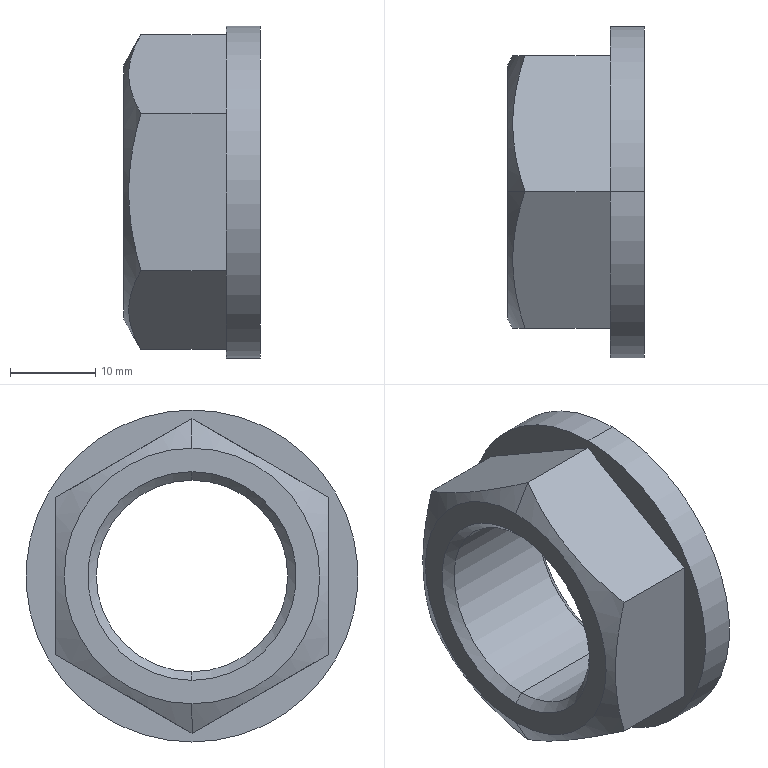Part | SolidWorks | features BaseBody 1 | 1 solid | 19 faces | box 16 x 39 x 39 mm | volume 8875 mm3 | plane 9 | cone 6 | cylinder 4 | commonest cylinder face diameters 22.5 x2 39 x2
STEP:
#1=CARTESIAN_POINT('',(-53.,0.,-19.5));
#2=VERTEX_POINT('',#1);
#3=CARTESIAN_POINT('',(-53.,0.,19.5));
#4=VERTEX_POINT('',#3);
#5=CARTESIAN_POINT('',(-53.,0.,0.));
#6=DIRECTION('',(1.,0.,0.));
#7=DIRECTION('',(0.,0.,-1.));
#8=AXIS2_PLACEMENT_3D('',#5,#6,#7);
#9=CIRCLE('',#8,19.5);
#10=EDGE_CURVE('',#2,#4,#9,.T.);
#11=ORIENTED_EDGE('',*,*,#10,.T.);
#12=CARTESIAN_POINT('',(-49.,0.,19.5));
#13=VERTEX_POINT('',#12);
#14=CARTESIAN_POINT('',(-53.,0.,19.5));
#15=DIRECTION('',(1.,0.,0.));
#16=VECTOR('',#15,1000.);
#17=LINE('',#14,#16);
#18=EDGE_CURVE('',#4,#13,#17,.T.);
#19=ORIENTED_EDGE('',*,*,#18,.T.);
#20=CARTESIAN_POINT('',(-49.,0.,-19.5));
#21=VERTEX_POINT('',#20);
#22=CARTESIAN_POINT('',(-49.,0.,0.));
#23=DIRECTION('',(1.,0.,0.));
#24=DIRECTION('',(0.,0.,-1.));
#25=AXIS2_PLACEMENT_3D('',#22,#23,#24);
#26=CIRCLE('',#25,19.5);
#27=EDGE_CURVE('',#21,#13,#26,.T.);
#28=ORIENTED_EDGE('',*,*,#27,.F.);
#29=CARTESIAN_POINT('',(-53.,0.,-19.5));
#30=DIRECTION('',(1.,0.,0.));
#31=VECTOR('',#30,1000.);
#32=LINE('',#29,#31);
#33=EDGE_CURVE('',#2,#21,#32,.T.);
#34=ORIENTED_EDGE('',*,*,#33,.F.);
#35=EDGE_LOOP('',(#11,#19,#28,#34));
#36=FACE_OUTER_BOUND('',#35,.T.);
#37=CARTESIAN_POINT('',(-53.,0.,0.));
#38=DIRECTION('',(1.,0.,0.));
#39=DIRECTION('',(0.,0.,-1.));
#40=AXIS2_PLACEMENT_3D('',#37,#38,#39);
#41=CYLINDRICAL_SURFACE('',#40,19.5);
#42=ADVANCED_FACE('',(#36),#41,.T.);
#43=CARTESIAN_POINT('',(-64.,0.,-11.25));
#44=VERTEX_POINT('',#43);
#45=CARTESIAN_POINT('',(-64.,0.,11.25));
#46=VERTEX_POINT('',#45);
#47=CARTESIAN_POINT('',(-64.,0.,0.));
#48=DIRECTION('',(-1.,0.,0.));
#49=DIRECTION('',(0.,0.,-1.));
#50=AXIS2_PLACEMENT_3D('',#47,#48,#49);
#51=CIRCLE('',#50,11.25);
#52=EDGE_CURVE('',#44,#46,#51,.T.);
#53=ORIENTED_EDGE('',*,*,#52,.F.);
#54=CARTESIAN_POINT('',(-65.,0.,-12.25));
#55=VERTEX_POINT('',#54);
#56=CARTESIAN_POINT('',(-65.,0.,-12.25));
#57=DIRECTION('',(-0.7071,0.,-0.7071));
#58=VECTOR('',#57,1000.);
#59=LINE('',#56,#58);
#60=EDGE_CURVE('',#44,#55,#59,.T.);
#61=ORIENTED_EDGE('',*,*,#60,.T.);
#62=CARTESIAN_POINT('',(-65.,0.,12.25));
#63=VERTEX_POINT('',#62);
#64=CARTESIAN_POINT('',(-65.,0.,0.));
#65=DIRECTION('',(1.,0.,0.));
#66=DIRECTION('',(0.,0.,-1.));
#67=AXIS2_PLACEMENT_3D('',#64,#65,#66);
#68=CIRCLE('',#67,12.25);
#69=EDGE_CURVE('',#63,#55,#68,.T.);
#70=ORIENTED_EDGE('',*,*,#69,.F.);
#71=CARTESIAN_POINT('',(-65.,0.,12.25));
#72=DIRECTION('',(-0.7071,0.,0.7071));
#73=VECTOR('',#72,1000.);
#74=LINE('',#71,#73);
#75=EDGE_CURVE('',#46,#63,#74,.T.);
#76=ORIENTED_EDGE('',*,*,#75,.F.);
#77=EDGE_LOOP('',(#53,#61,#70,#76));
#78=FACE_OUTER_BOUND('',#77,.T.);
#79=CARTESIAN_POINT('',(-65.,0.,0.));
#80=DIRECTION('',(-1.,0.,0.));
#81=DIRECTION('',(0.,0.,1.));
#82=AXIS2_PLACEMENT_3D('',#79,#80,#81);
#83=CONICAL_SURFACE('',#82,12.25,0.7854);
#84=ADVANCED_FACE('',(#78),#83,.F.);
#85=CARTESIAN_POINT('',(-50.,0.,11.25));
#86=VERTEX_POINT('',#85);
#87=CARTESIAN_POINT('',(-50.,0.,-11.25));
#88=VERTEX_POINT('',#87);
#89=CARTESIAN_POINT('',(-50.,0.,0.));
#90=DIRECTION('',(1.,0.,0.));
#91=DIRECTION('',(0.,0.,-1.));
#92=AXIS2_PLACEMENT_3D('',#89,#90,#91);
#93=CIRCLE('',#92,11.25);
#94=EDGE_CURVE('',#86,#88,#93,.T.);
#95=ORIENTED_EDGE('',*,*,#94,.F.);
#96=CARTESIAN_POINT('',(-49.,0.,12.25));
#97=VERTEX_POINT('',#96);
#98=CARTESIAN_POINT('',(-50.,0.,11.25));
#99=DIRECTION('',(0.7071,0.,0.7071));
#100=VECTOR('',#99,1000.);
#101=LINE('',#98,#100);
#102=EDGE_CURVE('',#86,#97,#101,.T.);
#103=ORIENTED_EDGE('',*,*,#102,.T.);
#104=CARTESIAN_POINT('',(-49.,0.,-12.25));
#105=VERTEX_POINT('',#104);
#106=CARTESIAN_POINT('',(-49.,0.,0.));
#107=DIRECTION('',(-1.,0.,0.));
#108=DIRECTION('',(0.,0.,-1.));
#109=AXIS2_PLACEMENT_3D('',#106,#107,#108);
#110=CIRCLE('',#109,12.25);
#111=EDGE_CURVE('',#105,#97,#110,.T.);
#112=ORIENTED_EDGE('',*,*,#111,.F.);
#113=CARTESIAN_POINT('',(-50.,0.,-11.25));
#114=DIRECTION('',(0.7071,0.,-0.7071));
#115=VECTOR('',#114,1000.);
#116=LINE('',#113,#115);
#117=EDGE_CURVE('',#88,#105,#116,.T.);
#118=ORIENTED_EDGE('',*,*,#117,.F.);
#119=EDGE_LOOP('',(#95,#103,#112,#118));
#120=FACE_OUTER_BOUND('',#119,.T.);
#121=CARTESIAN_POINT('',(-50.,0.,0.));
#122=DIRECTION('',(1.,0.,0.));
#123=DIRECTION('',(0.,0.,-1.));
#124=AXIS2_PLACEMENT_3D('',#121,#122,#123);
#125=CONICAL_SURFACE('',#124,11.25,0.7854);
#126=ADVANCED_FACE('',(#120),#125,.F.);
#127=CARTESIAN_POINT('',(-65.,0.,15.011));
#128=VERTEX_POINT('',#127);
#129=CARTESIAN_POINT('',(-65.,0.,-15.011));
#130=VERTEX_POINT('',#129);
#131=CARTESIAN_POINT('',(-65.,0.,0.));
#132=DIRECTION('',(-1.,0.,0.));
#133=DIRECTION('',(0.,0.,1.));
#134=AXIS2_PLACEMENT_3D('',#131,#132,#133);
#135=CIRCLE('',#134,15.011);
#136=EDGE_CURVE('',#128,#130,#135,.T.);
#137=ORIENTED_EDGE('',*,*,#136,.F.);
#138=CARTESIAN_POINT('',(-63.,0.,18.475));
#139=VERTEX_POINT('',#138);
#140=CARTESIAN_POINT('',(-65.,0.,15.011));
#141=DIRECTION('',(0.5,0.,0.866));
#142=VECTOR('',#141,1000.);
#143=LINE('',#140,#142);
#144=EDGE_CURVE('',#128,#139,#143,.T.);
#145=ORIENTED_EDGE('',*,*,#144,.T.);
#146=CARTESIAN_POINT('',(-63.,16.,9.238));
#147=VERTEX_POINT('',#146);
#148=CARTESIAN_POINT('',(-63.,0.,18.475));
#149=CARTESIAN_POINT('',(-63.435,1.306,17.721));
#150=CARTESIAN_POINT('',(-63.794,2.622,16.961));
#151=CARTESIAN_POINT('',(-64.291,5.281,15.426));
#152=CARTESIAN_POINT('',(-64.428,6.624,14.651));
#153=CARTESIAN_POINT('',(-64.43,8.665,13.473));
#154=CARTESIAN_POINT('',(-64.396,9.348,13.078));
#155=CARTESIAN_POINT('',(-64.266,10.7,12.298));
#156=CARTESIAN_POINT('',(-64.169,11.371,11.91));
#157=CARTESIAN_POINT('',(-63.796,13.373,10.754));
#158=CARTESIAN_POINT('',(-63.436,14.692,9.993));
#159=CARTESIAN_POINT('',(-63.,16.,9.238));
#160=B_SPLINE_CURVE_WITH_KNOTS('',3,(#148,#149,#150,#151,#152,#153,#154,#155,#156,#157,#158,#159),.UNSPECIFIED.,.F.,.F.,(4,2,2,2,2,4),(0.000000238,0.004665,0.00933,0.01166,0.01399,0.01866),.UNSPECIFIED.);
#161=EDGE_CURVE('',#139,#147,#160,.T.);
#162=ORIENTED_EDGE('',*,*,#161,.T.);
#163=CARTESIAN_POINT('',(-63.,16.,-9.238));
#164=VERTEX_POINT('',#163);
#165=CARTESIAN_POINT('',(-63.,16.,9.238));
#166=CARTESIAN_POINT('',(-63.217,16.,8.486));
#167=CARTESIAN_POINT('',(-63.416,16.,7.728));
#168=CARTESIAN_POINT('',(-63.769,16.,6.194));
#169=CARTESIAN_POINT('',(-63.922,16.,5.424));
#170=CARTESIAN_POINT('',(-64.295,16.,3.11));
#171=CARTESIAN_POINT('',(-64.429,16.,1.559));
#172=CARTESIAN_POINT('',(-64.429,16.,-0.7833));
#173=CARTESIAN_POINT('',(-64.396,16.,-1.566));
#174=CARTESIAN_POINT('',(-64.264,16.,-3.137));
#175=CARTESIAN_POINT('',(-64.166,16.,-3.918));
#176=CARTESIAN_POINT('',(-63.79,16.,-6.232));
#177=CARTESIAN_POINT('',(-63.431,16.,-7.744));
#178=CARTESIAN_POINT('',(-63.,16.,-9.238));
#179=B_SPLINE_CURVE_WITH_KNOTS('',3,(#165,#166,#167,#168,#169,#170,#171,#172,#173,#174,#175,#176,#177,#178),.UNSPECIFIED.,.F.,.F.,(4,2,2,2,2,2,4),(0.01639,0.01873,0.02107,0.02574,0.02808,0.03041,0.03509),.UNSPECIFIED.);
#180=EDGE_CURVE('',#147,#164,#179,.T.);
#181=ORIENTED_EDGE('',*,*,#180,.T.);
#182=CARTESIAN_POINT('',(-63.,0.,-18.475));
#183=VERTEX_POINT('',#182);
#184=CARTESIAN_POINT('',(-63.,16.,-9.238));
#185=CARTESIAN_POINT('',(-63.435,14.694,-9.992));
#186=CARTESIAN_POINT('',(-63.794,13.378,-10.751));
#187=CARTESIAN_POINT('',(-64.291,10.719,-12.287));
#188=CARTESIAN_POINT('',(-64.428,9.376,-13.062));
#189=CARTESIAN_POINT('',(-64.43,7.335,-14.24));
#190=CARTESIAN_POINT('',(-64.396,6.652,-14.635));
#191=CARTESIAN_POINT('',(-64.266,5.3,-15.415));
#192=CARTESIAN_POINT('',(-64.169,4.629,-15.803));
#193=CARTESIAN_POINT('',(-63.796,2.627,-16.959));
#194=CARTESIAN_POINT('',(-63.436,1.308,-17.72));
#195=CARTESIAN_POINT('',(-63.,0.,-18.475));
#196=B_SPLINE_CURVE_WITH_KNOTS('',3,(#184,#185,#186,#187,#188,#189,#190,#191,#192,#193,#194,#195),.UNSPECIFIED.,.F.,.F.,(4,2,2,2,2,4),(0.000000238,0.004665,0.00933,0.01166,0.01399,0.01866),.UNSPECIFIED.);
#197=EDGE_CURVE('',#164,#183,#196,.T.);
#198=ORIENTED_EDGE('',*,*,#197,.T.);
#199=CARTESIAN_POINT('',(-65.,0.,-15.011));
#200=DIRECTION('',(0.5,0.,-0.866));
#201=VECTOR('',#200,1000.);
#202=LINE('',#199,#201);
#203=EDGE_CURVE('',#130,#183,#202,.T.);
#204=ORIENTED_EDGE('',*,*,#203,.F.);
#205=EDGE_LOOP('',(#137,#145,#162,#181,#198,#204));
#206=FACE_OUTER_BOUND('',#205,.T.);
#207=CARTESIAN_POINT('',(-65.,0.,0.));
#208=DIRECTION('',(1.,0.,0.));
#209=DIRECTION('',(0.,0.,-1.));
#210=AXIS2_PLACEMENT_3D('',#207,#208,#209);
#211=CONICAL_SURFACE('',#210,15.011,1.047);
#212=ADVANCED_FACE('',(#206),#211,.T.);
#213=ORIENTED_EDGE('',*,*,#94,.T.);
#214=CARTESIAN_POINT('',(-49.,0.,-11.25));
#215=DIRECTION('',(-1.,0.,0.));
#216=VECTOR('',#215,1000.);
#217=LINE('',#214,#216);
#218=EDGE_CURVE('',#88,#44,#217,.T.);
#219=ORIENTED_EDGE('',*,*,#218,.T.);
#220=ORIENTED_EDGE('',*,*,#52,.T.);
#221=CARTESIAN_POINT('',(-49.,0.,11.25));
#222=DIRECTION('',(-1.,0.,0.));
#223=VECTOR('',#222,1000.);
#224=LINE('',#221,#223);
#225=EDGE_CURVE('',#86,#46,#224,.T.);
#226=ORIENTED_EDGE('',*,*,#225,.F.);
#227=EDGE_LOOP('',(#213,#219,#220,#226));
#228=FACE_OUTER_BOUND('',#227,.T.);
#229=CARTESIAN_POINT('',(-49.,0.,0.));
#230=DIRECTION('',(-1.,0.,0.));
#231=DIRECTION('',(0.,0.,1.));
#232=AXIS2_PLACEMENT_3D('',#229,#230,#231);
#233=CYLINDRICAL_SURFACE('',#232,11.25);
#234=ADVANCED_FACE('',(#228),#233,.F.);
#235=CARTESIAN_POINT('',(-53.,-16.,-9.238));
#236=VERTEX_POINT('',#235);
#237=CARTESIAN_POINT('',(-53.,0.,-18.475));
#238=VERTEX_POINT('',#237);
#239=CARTESIAN_POINT('',(-53.,-16.,-9.238));
#240=DIRECTION('',(0.,0.866,-0.5));
#241=VECTOR('',#240,1000.);
#242=LINE('',#239,#241);
#243=EDGE_CURVE('',#236,#238,#242,.T.);
#244=ORIENTED_EDGE('',*,*,#243,.F.);
#245=CARTESIAN_POINT('',(-63.,-16.,-9.238));
#246=VERTEX_POINT('',#245);
#247=CARTESIAN_POINT('',(-49.,-16.,-9.238));
#248=DIRECTION('',(-1.,0.,0.));
#249=VECTOR('',#248,1000.);
#250=LINE('',#247,#249);
#251=EDGE_CURVE('',#236,#246,#250,.T.);
#252=ORIENTED_EDGE('',*,*,#251,.T.);
#253=CARTESIAN_POINT('',(-63.,0.,-18.475));
#254=CARTESIAN_POINT('',(-63.435,-1.306,-17.721));
#255=CARTESIAN_POINT('',(-63.794,-2.622,-16.961));
#256=CARTESIAN_POINT('',(-64.291,-5.281,-15.426));
#257=CARTESIAN_POINT('',(-64.428,-6.624,-14.651));
#258=CARTESIAN_POINT('',(-64.43,-8.665,-13.473));
#259=CARTESIAN_POINT('',(-64.396,-9.348,-13.078));
#260=CARTESIAN_POINT('',(-64.266,-10.7,-12.298));
#261=CARTESIAN_POINT('',(-64.169,-11.371,-11.91));
#262=CARTESIAN_POINT('',(-63.796,-13.373,-10.754));
#263=CARTESIAN_POINT('',(-63.436,-14.692,-9.993));
#264=CARTESIAN_POINT('',(-63.,-16.,-9.238));
#265=B_SPLINE_CURVE_WITH_KNOTS('',3,(#253,#254,#255,#256,#257,#258,#259,#260,#261,#262,#263,#264),.UNSPECIFIED.,.F.,.F.,(4,2,2,2,2,4),(0.000000238,0.004665,0.00933,0.01166,0.01399,0.01866),.UNSPECIFIED.);
#266=EDGE_CURVE('',#183,#246,#265,.T.);
#267=ORIENTED_EDGE('',*,*,#266,.F.);
#268=CARTESIAN_POINT('',(-49.,0.,-18.475));
#269=DIRECTION('',(-1.,0.,0.));
#270=VECTOR('',#269,1000.);
#271=LINE('',#268,#270);
#272=EDGE_CURVE('',#238,#183,#271,.T.);
#273=ORIENTED_EDGE('',*,*,#272,.F.);
#274=EDGE_LOOP('',(#244,#252,#267,#273));
#275=FACE_OUTER_BOUND('',#274,.T.);
#276=CARTESIAN_POINT('',(-49.,-16.,-9.238));
#277=DIRECTION('',(0.,0.5,0.866));
#278=DIRECTION('',(0.,-0.866,0.5));
#279=AXIS2_PLACEMENT_3D('',#276,#277,#278);
#280=PLANE('',#279);
#281=ADVANCED_FACE('',(#275),#280,.F.);
#282=CARTESIAN_POINT('',(-53.,16.,-9.238));
#283=VERTEX_POINT('',#282);
#284=CARTESIAN_POINT('',(-53.,0.,-18.475));
#285=DIRECTION('',(0.,0.866,0.5));
#286=VECTOR('',#285,1000.);
#287=LINE('',#284,#286);
#288=EDGE_CURVE('',#238,#283,#287,.T.);
#289=ORIENTED_EDGE('',*,*,#288,.F.);
#290=ORIENTED_EDGE('',*,*,#272,.T.);
#291=ORIENTED_EDGE('',*,*,#197,.F.);
#292=CARTESIAN_POINT('',(-49.,16.,-9.238));
#293=DIRECTION('',(-1.,0.,0.));
#294=VECTOR('',#293,1000.);
#295=LINE('',#292,#294);
#296=EDGE_CURVE('',#283,#164,#295,.T.);
#297=ORIENTED_EDGE('',*,*,#296,.F.);
#298=EDGE_LOOP('',(#289,#290,#291,#297));
#299=FACE_OUTER_BOUND('',#298,.T.);
#300=CARTESIAN_POINT('',(-49.,0.,-18.475));
#301=DIRECTION('',(0.,-0.5,0.866));
#302=DIRECTION('',(0.,-0.866,-0.5));
#303=AXIS2_PLACEMENT_3D('',#300,#301,#302);
#304=PLANE('',#303);
#305=ADVANCED_FACE('',(#299),#304,.F.);
#306=CARTESIAN_POINT('',(-53.,16.,9.238));
#307=VERTEX_POINT('',#306);
#308=CARTESIAN_POINT('',(-53.,16.,-9.238));
#309=DIRECTION('',(0.,0.,1.));
#310=VECTOR('',#309,1000.);
#311=LINE('',#308,#310);
#312=EDGE_CURVE('',#283,#307,#311,.T.);
#313=ORIENTED_EDGE('',*,*,#312,.F.);
#314=ORIENTED_EDGE('',*,*,#296,.T.);
#315=ORIENTED_EDGE('',*,*,#180,.F.);
#316=CARTESIAN_POINT('',(-49.,16.,9.238));
#317=DIRECTION('',(-1.,0.,0.));
#318=VECTOR('',#317,1000.);
#319=LINE('',#316,#318);
#320=EDGE_CURVE('',#307,#147,#319,.T.);
#321=ORIENTED_EDGE('',*,*,#320,.F.);
#322=EDGE_LOOP('',(#313,#314,#315,#321));
#323=FACE_OUTER_BOUND('',#322,.T.);
#324=CARTESIAN_POINT('',(-49.,16.,-9.238));
#325=DIRECTION('',(0.,-1.,0.));
#326=DIRECTION('',(-1.,0.,0.));
#327=AXIS2_PLACEMENT_3D('',#324,#325,#326);
#328=PLANE('',#327);
#329=ADVANCED_FACE('',(#323),#328,.F.);
#330=CARTESIAN_POINT('',(-53.,0.,18.475));
#331=VERTEX_POINT('',#330);
#332=CARTESIAN_POINT('',(-53.,16.,9.238));
#333=DIRECTION('',(0.,-0.866,0.5));
#334=VECTOR('',#333,1000.);
#335=LINE('',#332,#334);
#336=EDGE_CURVE('',#307,#331,#335,.T.);
#337=ORIENTED_EDGE('',*,*,#336,.F.);
#338=ORIENTED_EDGE('',*,*,#320,.T.);
#339=ORIENTED_EDGE('',*,*,#161,.F.);
#340=CARTESIAN_POINT('',(-49.,0.,18.475));
#341=DIRECTION('',(-1.,0.,0.));
#342=VECTOR('',#341,1000.);
#343=LINE('',#340,#342);
#344=EDGE_CURVE('',#331,#139,#343,.T.);
#345=ORIENTED_EDGE('',*,*,#344,.F.);
#346=EDGE_LOOP('',(#337,#338,#339,#345));
#347=FACE_OUTER_BOUND('',#346,.T.);
#348=CARTESIAN_POINT('',(-49.,16.,9.238));
#349=DIRECTION('',(0.,-0.5,-0.866));
#350=DIRECTION('',(0.,0.866,-0.5));
#351=AXIS2_PLACEMENT_3D('',#348,#349,#350);
#352=PLANE('',#351);
#353=ADVANCED_FACE('',(#347),#352,.F.);
#354=CARTESIAN_POINT('',(-53.,-16.,9.238));
#355=VERTEX_POINT('',#354);
#356=CARTESIAN_POINT('',(-53.,0.,18.475));
#357=DIRECTION('',(0.,-0.866,-0.5));
#358=VECTOR('',#357,1000.);
#359=LINE('',#356,#358);
#360=EDGE_CURVE('',#331,#355,#359,.T.);
#361=ORIENTED_EDGE('',*,*,#360,.F.);
#362=ORIENTED_EDGE('',*,*,#344,.T.);
#363=CARTESIAN_POINT('',(-63.,-16.,9.238));
#364=VERTEX_POINT('',#363);
#365=CARTESIAN_POINT('',(-63.,-16.,9.238));
#366=CARTESIAN_POINT('',(-63.435,-14.694,9.992));
#367=CARTESIAN_POINT('',(-63.794,-13.378,10.751));
#368=CARTESIAN_POINT('',(-64.291,-10.719,12.287));
#369=CARTESIAN_POINT('',(-64.428,-9.376,13.062));
#370=CARTESIAN_POINT('',(-64.43,-7.335,14.24));
#371=CARTESIAN_POINT('',(-64.396,-6.652,14.635));
#372=CARTESIAN_POINT('',(-64.266,-5.3,15.415));
#373=CARTESIAN_POINT('',(-64.169,-4.629,15.803));
#374=CARTESIAN_POINT('',(-63.796,-2.627,16.959));
#375=CARTESIAN_POINT('',(-63.436,-1.308,17.72));
#376=CARTESIAN_POINT('',(-63.,0.,18.475));
#377=B_SPLINE_CURVE_WITH_KNOTS('',3,(#365,#366,#367,#368,#369,#370,#371,#372,#373,#374,#375,#376),.UNSPECIFIED.,.F.,.F.,(4,2,2,2,2,4),(0.000000238,0.004665,0.00933,0.01166,0.01399,0.01866),.UNSPECIFIED.);
#378=EDGE_CURVE('',#364,#139,#377,.T.);
#379=ORIENTED_EDGE('',*,*,#378,.F.);
#380=CARTESIAN_POINT('',(-49.,-16.,9.238));
#381=DIRECTION('',(-1.,0.,0.));
#382=VECTOR('',#381,1000.);
#383=LINE('',#380,#382);
#384=EDGE_CURVE('',#355,#364,#383,.T.);
#385=ORIENTED_EDGE('',*,*,#384,.F.);
#386=EDGE_LOOP('',(#361,#362,#379,#385));
#387=FACE_OUTER_BOUND('',#386,.T.);
#388=CARTESIAN_POINT('',(-49.,0.,18.475));
#389=DIRECTION('',(0.,0.5,-0.866));
#390=DIRECTION('',(0.,0.866,0.5));
#391=AXIS2_PLACEMENT_3D('',#388,#389,#390);
#392=PLANE('',#391);
#393=ADVANCED_FACE('',(#387),#392,.F.);
#394=CARTESIAN_POINT('',(-53.,-16.,9.238));
#395=DIRECTION('',(0.,0.,-1.));
#396=VECTOR('',#395,1000.);
#397=LINE('',#394,#396);
#398=EDGE_CURVE('',#355,#236,#397,.T.);
#399=ORIENTED_EDGE('',*,*,#398,.F.);
#400=ORIENTED_EDGE('',*,*,#384,.T.);
#401=CARTESIAN_POINT('',(-63.,-16.,-9.238));
#402=CARTESIAN_POINT('',(-63.431,-16.,-7.744));
#403=CARTESIAN_POINT('',(-63.79,-16.,-6.232));
#404=CARTESIAN_POINT('',(-64.166,-16.,-3.918));
#405=CARTESIAN_POINT('',(-64.264,-16.,-3.137));
#406=CARTESIAN_POINT('',(-64.396,-16.,-1.566));
#407=CARTESIAN_POINT('',(-64.429,-16.,-0.7833));
#408=CARTESIAN_POINT('',(-64.429,-16.,1.559));
#409=CARTESIAN_POINT('',(-64.295,-16.,3.11));
#410=CARTESIAN_POINT('',(-63.922,-16.,5.424));
#411=CARTESIAN_POINT('',(-63.769,-16.,6.194));
#412=CARTESIAN_POINT('',(-63.416,-16.,7.728));
#413=CARTESIAN_POINT('',(-63.217,-16.,8.486));
#414=CARTESIAN_POINT('',(-63.,-16.,9.238));
#415=B_SPLINE_CURVE_WITH_KNOTS('',3,(#401,#402,#403,#404,#405,#406,#407,#408,#409,#410,#411,#412,#413,#414),.UNSPECIFIED.,.F.,.F.,(4,2,2,2,2,2,4),(0.006866,0.01153,0.01386,0.01619,0.02085,0.02318,0.02551),.UNSPECIFIED.);
#416=EDGE_CURVE('',#246,#364,#415,.T.);
#417=ORIENTED_EDGE('',*,*,#416,.F.);
#418=ORIENTED_EDGE('',*,*,#251,.F.);
#419=EDGE_LOOP('',(#399,#400,#417,#418));
#420=FACE_OUTER_BOUND('',#419,.T.);
#421=CARTESIAN_POINT('',(-49.,-16.,9.238));
#422=DIRECTION('',(0.,1.,0.));
#423=DIRECTION('',(0.,0.,1.));
#424=AXIS2_PLACEMENT_3D('',#421,#422,#423);
#425=PLANE('',#424);
#426=ADVANCED_FACE('',(#420),#425,.F.);
#427=ORIENTED_EDGE('',*,*,#69,.T.);
#428=CARTESIAN_POINT('',(-65.,0.,0.));
#429=DIRECTION('',(1.,0.,0.));
#430=DIRECTION('',(0.,0.,-1.));
#431=AXIS2_PLACEMENT_3D('',#428,#429,#430);
#432=CIRCLE('',#431,12.25);
#433=EDGE_CURVE('',#55,#63,#432,.T.);
#434=ORIENTED_EDGE('',*,*,#433,.T.);
#435=EDGE_LOOP('',(#427,#434));
#436=FACE_BOUND('',#435,.T.);
#437=CARTESIAN_POINT('',(-65.,0.,0.));
#438=DIRECTION('',(-1.,0.,0.));
#439=DIRECTION('',(0.,0.,1.));
#440=AXIS2_PLACEMENT_3D('',#437,#438,#439);
#441=CIRCLE('',#440,15.011);
#442=EDGE_CURVE('',#130,#128,#441,.T.);
#443=ORIENTED_EDGE('',*,*,#442,.T.);
#444=ORIENTED_EDGE('',*,*,#136,.T.);
#445=EDGE_LOOP('',(#443,#444));
#446=FACE_OUTER_BOUND('',#445,.T.);
#447=CARTESIAN_POINT('',(-65.,0.,-18.475));
#448=DIRECTION('',(1.,0.,0.));
#449=DIRECTION('',(0.,0.,-1.));
#450=AXIS2_PLACEMENT_3D('',#447,#448,#449);
#451=PLANE('',#450);
#452=ADVANCED_FACE('',(#436,#446),#451,.F.);
#453=ORIENTED_EDGE('',*,*,#111,.T.);
#454=CARTESIAN_POINT('',(-49.,0.,0.));
#455=DIRECTION('',(-1.,0.,0.));
#456=DIRECTION('',(0.,0.,-1.));
#457=AXIS2_PLACEMENT_3D('',#454,#455,#456);
#458=CIRCLE('',#457,12.25);
#459=EDGE_CURVE('',#97,#105,#458,.T.);
#460=ORIENTED_EDGE('',*,*,#459,.T.);
#461=EDGE_LOOP('',(#453,#460));
#462=FACE_BOUND('',#461,.T.);
#463=ORIENTED_EDGE('',*,*,#27,.T.);
#464=CARTESIAN_POINT('',(-49.,0.,0.));
#465=DIRECTION('',(1.,0.,0.));
#466=DIRECTION('',(0.,0.,-1.));
#467=AXIS2_PLACEMENT_3D('',#464,#465,#466);
#468=CIRCLE('',#467,19.5);
#469=EDGE_CURVE('',#13,#21,#468,.T.);
#470=ORIENTED_EDGE('',*,*,#469,.T.);
#471=EDGE_LOOP('',(#463,#470));
#472=FACE_OUTER_BOUND('',#471,.T.);
#473=CARTESIAN_POINT('',(-49.,0.,-18.475));
#474=DIRECTION('',(1.,0.,0.));
#475=DIRECTION('',(0.,0.,-1.));
#476=AXIS2_PLACEMENT_3D('',#473,#474,#475);
#477=PLANE('',#476);
#478=ADVANCED_FACE('',(#462,#472),#477,.T.);
#479=ORIENTED_EDGE('',*,*,#218,.F.);
#480=CARTESIAN_POINT('',(-50.,0.,0.));
#481=DIRECTION('',(1.,0.,0.));
#482=DIRECTION('',(0.,0.,-1.));
#483=AXIS2_PLACEMENT_3D('',#480,#481,#482);
#484=CIRCLE('',#483,11.25);
#485=EDGE_CURVE('',#88,#86,#484,.T.);
#486=ORIENTED_EDGE('',*,*,#485,.T.);
#487=ORIENTED_EDGE('',*,*,#225,.T.);
#488=CARTESIAN_POINT('',(-64.,0.,0.));
#489=DIRECTION('',(-1.,0.,0.));
#490=DIRECTION('',(0.,0.,-1.));
#491=AXIS2_PLACEMENT_3D('',#488,#489,#490);
#492=CIRCLE('',#491,11.25);
#493=EDGE_CURVE('',#46,#44,#492,.T.);
#494=ORIENTED_EDGE('',*,*,#493,.T.);
#495=EDGE_LOOP('',(#479,#486,#487,#494));
#496=FACE_OUTER_BOUND('',#495,.T.);
#497=CARTESIAN_POINT('',(-49.,0.,0.));
#498=DIRECTION('',(-1.,0.,0.));
#499=DIRECTION('',(0.,0.,1.));
#500=AXIS2_PLACEMENT_3D('',#497,#498,#499);
#501=CYLINDRICAL_SURFACE('',#500,11.25);
#502=ADVANCED_FACE('',(#496),#501,.F.);
#503=ORIENTED_EDGE('',*,*,#144,.F.);
#504=ORIENTED_EDGE('',*,*,#442,.F.);
#505=ORIENTED_EDGE('',*,*,#203,.T.);
#506=ORIENTED_EDGE('',*,*,#266,.T.);
#507=ORIENTED_EDGE('',*,*,#416,.T.);
#508=ORIENTED_EDGE('',*,*,#378,.T.);
#509=EDGE_LOOP('',(#503,#504,#505,#506,#507,#508));
#510=FACE_OUTER_BOUND('',#509,.T.);
#511=CARTESIAN_POINT('',(-65.,0.,0.));
#512=DIRECTION('',(1.,0.,0.));
#513=DIRECTION('',(0.,0.,-1.));
#514=AXIS2_PLACEMENT_3D('',#511,#512,#513);
#515=CONICAL_SURFACE('',#514,15.011,1.047);
#516=ADVANCED_FACE('',(#510),#515,.T.);
#517=ORIENTED_EDGE('',*,*,#102,.F.);
#518=ORIENTED_EDGE('',*,*,#485,.F.);
#519=ORIENTED_EDGE('',*,*,#117,.T.);
#520=ORIENTED_EDGE('',*,*,#459,.F.);
#521=EDGE_LOOP('',(#517,#518,#519,#520));
#522=FACE_OUTER_BOUND('',#521,.T.);
#523=CARTESIAN_POINT('',(-50.,0.,0.));
#524=DIRECTION('',(1.,0.,0.));
#525=DIRECTION('',(0.,0.,-1.));
#526=AXIS2_PLACEMENT_3D('',#523,#524,#525);
#527=CONICAL_SURFACE('',#526,11.25,0.7854);
#528=ADVANCED_FACE('',(#522),#527,.F.);
#529=ORIENTED_EDGE('',*,*,#60,.F.);
#530=ORIENTED_EDGE('',*,*,#493,.F.);
#531=ORIENTED_EDGE('',*,*,#75,.T.);
#532=ORIENTED_EDGE('',*,*,#433,.F.);
#533=EDGE_LOOP('',(#529,#530,#531,#532));
#534=FACE_OUTER_BOUND('',#533,.T.);
#535=CARTESIAN_POINT('',(-65.,0.,0.));
#536=DIRECTION('',(-1.,0.,0.));
#537=DIRECTION('',(0.,0.,1.));
#538=AXIS2_PLACEMENT_3D('',#535,#536,#537);
#539=CONICAL_SURFACE('',#538,12.25,0.7854);
#540=ADVANCED_FACE('',(#534),#539,.F.);
#541=ORIENTED_EDGE('',*,*,#18,.F.);
#542=CARTESIAN_POINT('',(-53.,0.,0.));
#543=DIRECTION('',(1.,0.,0.));
#544=DIRECTION('',(0.,0.,-1.));
#545=AXIS2_PLACEMENT_3D('',#542,#543,#544);
#546=CIRCLE('',#545,19.5);
#547=EDGE_CURVE('',#4,#2,#546,.T.);
#548=ORIENTED_EDGE('',*,*,#547,.T.);
#549=ORIENTED_EDGE('',*,*,#33,.T.);
#550=ORIENTED_EDGE('',*,*,#469,.F.);
#551=EDGE_LOOP('',(#541,#548,#549,#550));
#552=FACE_OUTER_BOUND('',#551,.T.);
#553=CARTESIAN_POINT('',(-53.,0.,0.));
#554=DIRECTION('',(1.,0.,0.));
#555=DIRECTION('',(0.,0.,-1.));
#556=AXIS2_PLACEMENT_3D('',#553,#554,#555);
#557=CYLINDRICAL_SURFACE('',#556,19.5);
#558=ADVANCED_FACE('',(#552),#557,.T.);
#559=ORIENTED_EDGE('',*,*,#398,.T.);
#560=ORIENTED_EDGE('',*,*,#243,.T.);
#561=ORIENTED_EDGE('',*,*,#288,.T.);
#562=ORIENTED_EDGE('',*,*,#312,.T.);
#563=ORIENTED_EDGE('',*,*,#336,.T.);
#564=ORIENTED_EDGE('',*,*,#360,.T.);
#565=EDGE_LOOP('',(#559,#560,#561,#562,#563,#564));
#566=FACE_BOUND('',#565,.T.);
#567=ORIENTED_EDGE('',*,*,#10,.F.);
#568=ORIENTED_EDGE('',*,*,#547,.F.);
#569=EDGE_LOOP('',(#567,#568));
#570=FACE_OUTER_BOUND('',#569,.T.);
#571=CARTESIAN_POINT('',(-53.,0.,0.));
#572=DIRECTION('',(1.,0.,0.));
#573=DIRECTION('',(0.,0.,-1.));
#574=AXIS2_PLACEMENT_3D('',#571,#572,#573);
#575=PLANE('',#574);
#576=ADVANCED_FACE('',(#566,#570),#575,.F.);
#577=CLOSED_SHELL('',(#42,#84,#126,#212,#234,#281,#305,#329,#353,#393,#426,#452,#478,#502,#516,#528,#540,#558,#576));
#578=MANIFOLD_SOLID_BREP('',#577);
#579=CARTESIAN_POINT('',(0.,0.,0.));
#580=DIRECTION('',(0.,0.,1.));
#581=DIRECTION('',(1.,0.,0.));
#582=AXIS2_PLACEMENT_3D('',#579,#580,#581);
#583=(LENGTH_UNIT()NAMED_UNIT(*)SI_UNIT(.MILLI.,.METRE.));
#584=UNCERTAINTY_MEASURE_WITH_UNIT(LENGTH_MEASURE(0.00001),#583,'','');
#585=(NAMED_UNIT(*)PLANE_ANGLE_UNIT()SI_UNIT($,.RADIAN.));
#586=(NAMED_UNIT(*)SI_UNIT($,.STERADIAN.)SOLID_ANGLE_UNIT());
#587=(GEOMETRIC_REPRESENTATION_CONTEXT(3)GLOBAL_UNCERTAINTY_ASSIGNED_CONTEXT((#584))GLOBAL_UNIT_ASSIGNED_CONTEXT((#583,#585,#586))REPRESENTATION_CONTEXT('',''));
#588=ADVANCED_BREP_SHAPE_REPRESENTATION('',(#578,#582),#587);